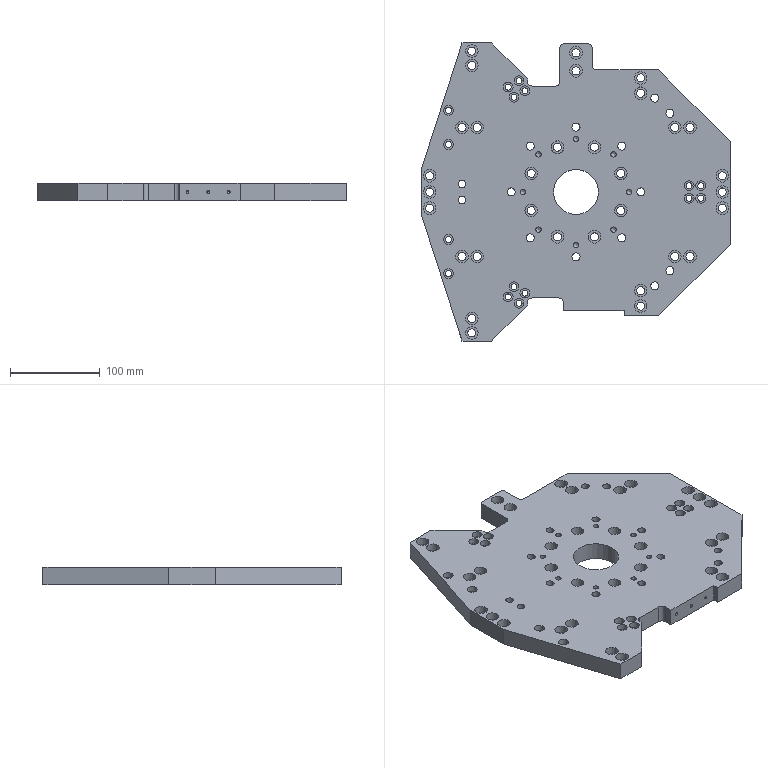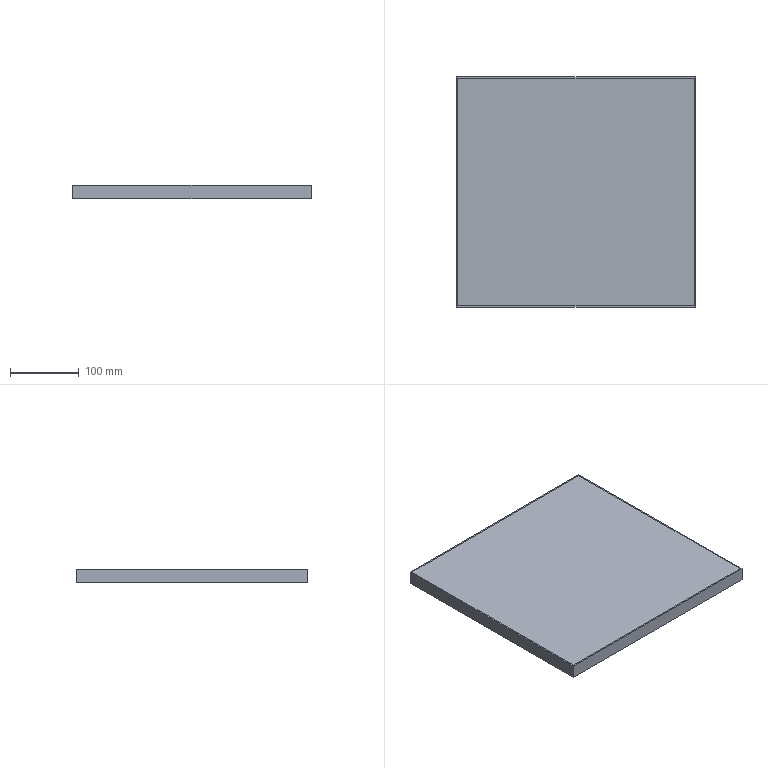CAM job | NX | 3-axis milling, drilling | part box 344 x 332 x 20 mm | stock box 348 x 336 x 20 mm
Tools:
number,name,description,diameter,corner_radius,flute_length,length,flutes
11,ZXZ,Milling Tool-5 Parameters,6.0,0.0,50.0,75.0,2
16,6.0ZT,Drilling Tool,6.0,0.0,35.0,50.0,2
19,9.0ZT,Drilling Tool,9.0,0.0,35.0,50.0,2
17,6.6ZT,Drilling Tool,6.6,0.0,35.0,50.0,2
10,D10,Milling Tool-5 Parameters,10.0,0.0,50.0,75.0,2
6,D6,Milling Tool-5 Parameters,6.0,0.0,50.0,75.0,2
9,D10JING,Milling Tool-5 Parameters,10.0,0.0,50.0,75.0,2
7,D6A45,Milling Tool-5 Parameters,6.0,0.0,3.0,3.0,2
18,8.5ZT,Drilling Tool,8.5,0.0,35.0,50.0,2
Operations:
program,operation,operation_type,tool,method,geometry_group,spindle_rpm,surface_speed,feed_per_tooth,feed_cut,feed_plunge,cut_length_mm,path_length_mm,cut_time_min,machine_time_min
1压左右,DRILLING,Operation,ZXZ,METHOD,A,3000.0,56.0,0.0417,250.0,0.0,284.0,2823.089,1.136,1.39
1压左右,DRILLING_COPY,Operation,6.0ZT,METHOD,A,2000.0,37.0,0.045,180.0,0.0,158.421,815.971,0.8801,0.9459
1压左右,DRILLING_COPY_COPY,Operation,9.0ZT,METHOD,A,1000.0,28.0,0.09,180.0,0.0,1174.97,4331.562,6.528,6.843
1压左右,DRILLING_COPY_COPY_COPY,Operation,9.0ZT,METHOD,A,1000.0,28.0,0.09,180.0,0.0,26.704,213.408,0.1484,0.167
1压左右,DRILLING_COPY_COPY_COPY_COPY,Operation,8.5ZT,METHOD,A,1000.0,28.0,0.09,180.0,0.0,53.107,287.266,0.295,0.3185
1压左右,DRILLING_COPY_COPY_1,Operation,6.6ZT,METHOD,A,2000.0,37.0,0.045,180.0,0.0,415.725,1698.805,2.31,2.438
1压左右,HOLE_MILLING,CylinderMilling,D10,METHOD,A,3200.0,100.0,0.3438,2200.0,100.0,20255.431,26988.959,9.207,9.88
1压左右,HOLE_MILLING_COPY_1,CylinderMilling,D10,METHOD,A,3200.0,100.0,0.3438,2200.0,100.0,7456.676,7636.176,3.389,3.407
1压左右,ZLEVEL_PROFILE,ZLevelMilling,D10,METHOD,A,2200.0,69.0,0.5,2200.0,100.0,47234.174,47957.101,21.47,21.542
1压左右,HOLE_MILLING_COPY,CylinderMilling,D6,METHOD,A,4000.0,75.0,0.2062,1650.0,100.0,19226.929,22553.944,11.653,11.985
1压左右,ZLEVEL_PROFILE_COPY,ZLevelMilling,D10JING,METHOD,A,5000.0,157.0,0.12,1200.0,100.0,497.815,1221.176,0.4148,0.4872
1压左右,ZLEVEL_PROFILE_COPY_COPY,ZLevelMilling,D6A45,METHOD,A,7500.0,141.0,0.08,1200.0,100.0,3419.117,27241.564,2.849,5.231
1压左右,刀补9,ZLevelMilling,D10JING,METHOD,A,5000.0,157.0,0.12,1200.0,100.0,145.133,339.133,0.1209,0.1403
2压前后,ZLEVEL_PROFILE_COPY_1,ZLevelMilling,D10,METHOD,A,2200.0,69.0,0.5,2200.0,100.0,77881.521,78385.218,35.401,35.451
2压前后,ZLEVEL_PROFILE_COPY_COPY_1,ZLevelMilling,D10JING,METHOD,A,5000.0,157.0,0.12,1200.0,100.0,834.693,1345.628,0.6956,0.7467
2压前后,ZLEVEL_PROFILE_COPY_COPY_COPY,ZLevelMilling,D6A45,METHOD,A,7500.0,141.0,0.08,1200.0,100.0,811.598,1459.996,0.6763,0.7412
2夹夹着做,HOLE_MILLING_COPY_2,CylinderMilling,D10,METHOD,B,3200.0,100.0,0.3438,2200.0,100.0,6738.857,9392.467,3.063,3.329
2夹夹着做,ZLEVEL_PROFILE_COPY_COPY_COPY_1,ZLevelMilling,D6A45,METHOD,B,7500.0,141.0,0.08,1200.0,100.0,3498.013,24466.361,2.915,5.012